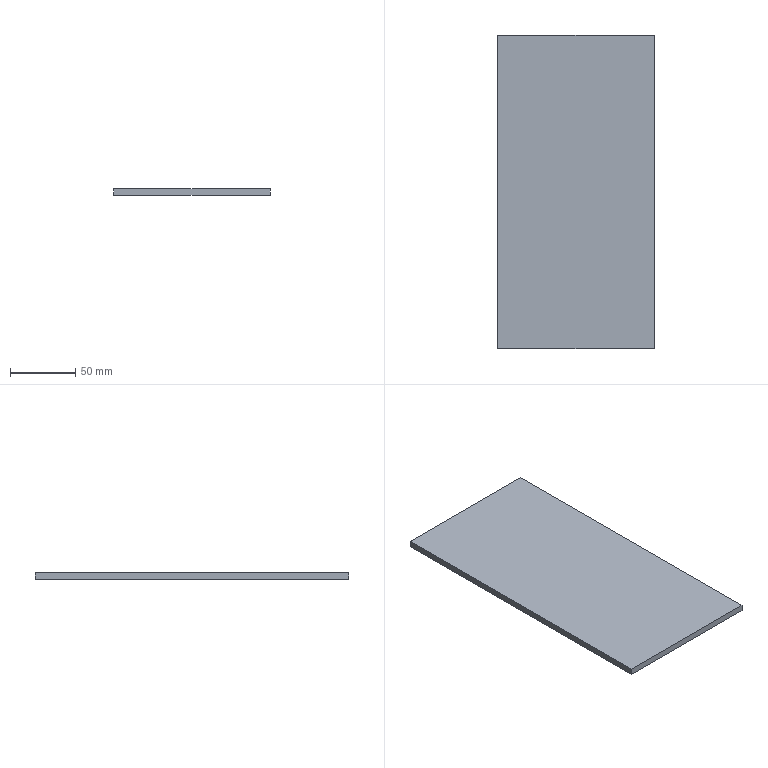Part | SolidWorks | features Extrusion 1 | 1 solid | 6 faces | box 120 x 240 x 5 mm | volume 144000 mm3 | plane 6
STEP:
#1=CARTESIAN_POINT('',(16.745,0.,0.));
#2=VERTEX_POINT('',#1);
#3=CARTESIAN_POINT('',(136.745,0.,0.));
#4=VERTEX_POINT('',#3);
#5=CARTESIAN_POINT('',(136.745,0.,0.));
#6=DIRECTION('',(1.,0.,0.));
#7=VECTOR('',#6,1000.);
#8=LINE('',#5,#7);
#9=EDGE_CURVE('',#2,#4,#8,.T.);
#10=ORIENTED_EDGE('',*,*,#9,.T.);
#11=CARTESIAN_POINT('',(136.745,0.,5.));
#12=VERTEX_POINT('',#11);
#13=CARTESIAN_POINT('',(136.745,0.,5.));
#14=DIRECTION('',(0.,0.,-1.));
#15=VECTOR('',#14,1000.);
#16=LINE('',#13,#15);
#17=EDGE_CURVE('',#12,#4,#16,.T.);
#18=ORIENTED_EDGE('',*,*,#17,.F.);
#19=CARTESIAN_POINT('',(16.745,0.,5.));
#20=VERTEX_POINT('',#19);
#21=CARTESIAN_POINT('',(136.745,0.,5.));
#22=DIRECTION('',(1.,0.,0.));
#23=VECTOR('',#22,1000.);
#24=LINE('',#21,#23);
#25=EDGE_CURVE('',#20,#12,#24,.T.);
#26=ORIENTED_EDGE('',*,*,#25,.F.);
#27=CARTESIAN_POINT('',(16.745,0.,5.));
#28=DIRECTION('',(0.,0.,-1.));
#29=VECTOR('',#28,1000.);
#30=LINE('',#27,#29);
#31=EDGE_CURVE('',#20,#2,#30,.T.);
#32=ORIENTED_EDGE('',*,*,#31,.T.);
#33=EDGE_LOOP('',(#10,#18,#26,#32));
#34=FACE_OUTER_BOUND('',#33,.T.);
#35=CARTESIAN_POINT('',(136.745,0.,5.));
#36=DIRECTION('',(0.,1.,0.));
#37=DIRECTION('',(0.,0.,1.));
#38=AXIS2_PLACEMENT_3D('',#35,#36,#37);
#39=PLANE('',#38);
#40=ADVANCED_FACE('',(#34),#39,.F.);
#41=CARTESIAN_POINT('',(136.745,240.,0.));
#42=VERTEX_POINT('',#41);
#43=CARTESIAN_POINT('',(136.745,240.,0.));
#44=DIRECTION('',(0.,1.,0.));
#45=VECTOR('',#44,1000.);
#46=LINE('',#43,#45);
#47=EDGE_CURVE('',#4,#42,#46,.T.);
#48=ORIENTED_EDGE('',*,*,#47,.T.);
#49=CARTESIAN_POINT('',(136.745,240.,5.));
#50=VERTEX_POINT('',#49);
#51=CARTESIAN_POINT('',(136.745,240.,5.));
#52=DIRECTION('',(0.,0.,-1.));
#53=VECTOR('',#52,1000.);
#54=LINE('',#51,#53);
#55=EDGE_CURVE('',#50,#42,#54,.T.);
#56=ORIENTED_EDGE('',*,*,#55,.F.);
#57=CARTESIAN_POINT('',(136.745,240.,5.));
#58=DIRECTION('',(0.,1.,0.));
#59=VECTOR('',#58,1000.);
#60=LINE('',#57,#59);
#61=EDGE_CURVE('',#12,#50,#60,.T.);
#62=ORIENTED_EDGE('',*,*,#61,.F.);
#63=ORIENTED_EDGE('',*,*,#17,.T.);
#64=EDGE_LOOP('',(#48,#56,#62,#63));
#65=FACE_OUTER_BOUND('',#64,.T.);
#66=CARTESIAN_POINT('',(136.745,240.,5.));
#67=DIRECTION('',(-1.,0.,0.));
#68=DIRECTION('',(0.,0.,1.));
#69=AXIS2_PLACEMENT_3D('',#66,#67,#68);
#70=PLANE('',#69);
#71=ADVANCED_FACE('',(#65),#70,.F.);
#72=CARTESIAN_POINT('',(16.745,240.,0.));
#73=VERTEX_POINT('',#72);
#74=CARTESIAN_POINT('',(16.745,240.,0.));
#75=DIRECTION('',(-1.,0.,0.));
#76=VECTOR('',#75,1000.);
#77=LINE('',#74,#76);
#78=EDGE_CURVE('',#42,#73,#77,.T.);
#79=ORIENTED_EDGE('',*,*,#78,.T.);
#80=CARTESIAN_POINT('',(16.745,240.,5.));
#81=VERTEX_POINT('',#80);
#82=CARTESIAN_POINT('',(16.745,240.,5.));
#83=DIRECTION('',(0.,0.,-1.));
#84=VECTOR('',#83,1000.);
#85=LINE('',#82,#84);
#86=EDGE_CURVE('',#81,#73,#85,.T.);
#87=ORIENTED_EDGE('',*,*,#86,.F.);
#88=CARTESIAN_POINT('',(16.745,240.,5.));
#89=DIRECTION('',(-1.,0.,0.));
#90=VECTOR('',#89,1000.);
#91=LINE('',#88,#90);
#92=EDGE_CURVE('',#50,#81,#91,.T.);
#93=ORIENTED_EDGE('',*,*,#92,.F.);
#94=ORIENTED_EDGE('',*,*,#55,.T.);
#95=EDGE_LOOP('',(#79,#87,#93,#94));
#96=FACE_OUTER_BOUND('',#95,.T.);
#97=CARTESIAN_POINT('',(16.745,240.,5.));
#98=DIRECTION('',(0.,-1.,0.));
#99=DIRECTION('',(0.,0.,-1.));
#100=AXIS2_PLACEMENT_3D('',#97,#98,#99);
#101=PLANE('',#100);
#102=ADVANCED_FACE('',(#96),#101,.F.);
#103=CARTESIAN_POINT('',(16.745,0.,0.));
#104=DIRECTION('',(0.,-1.,0.));
#105=VECTOR('',#104,1000.);
#106=LINE('',#103,#105);
#107=EDGE_CURVE('',#73,#2,#106,.T.);
#108=ORIENTED_EDGE('',*,*,#107,.T.);
#109=ORIENTED_EDGE('',*,*,#31,.F.);
#110=CARTESIAN_POINT('',(16.745,0.,5.));
#111=DIRECTION('',(0.,-1.,0.));
#112=VECTOR('',#111,1000.);
#113=LINE('',#110,#112);
#114=EDGE_CURVE('',#81,#20,#113,.T.);
#115=ORIENTED_EDGE('',*,*,#114,.F.);
#116=ORIENTED_EDGE('',*,*,#86,.T.);
#117=EDGE_LOOP('',(#108,#109,#115,#116));
#118=FACE_OUTER_BOUND('',#117,.T.);
#119=CARTESIAN_POINT('',(16.745,0.,5.));
#120=DIRECTION('',(1.,0.,0.));
#121=DIRECTION('',(0.,0.,-1.));
#122=AXIS2_PLACEMENT_3D('',#119,#120,#121);
#123=PLANE('',#122);
#124=ADVANCED_FACE('',(#118),#123,.F.);
#125=ORIENTED_EDGE('',*,*,#25,.T.);
#126=ORIENTED_EDGE('',*,*,#61,.T.);
#127=ORIENTED_EDGE('',*,*,#92,.T.);
#128=ORIENTED_EDGE('',*,*,#114,.T.);
#129=EDGE_LOOP('',(#125,#126,#127,#128));
#130=FACE_OUTER_BOUND('',#129,.T.);
#131=CARTESIAN_POINT('',(0.,0.,5.));
#132=DIRECTION('',(0.,0.,-1.));
#133=DIRECTION('',(-1.,0.,0.));
#134=AXIS2_PLACEMENT_3D('',#131,#132,#133);
#135=PLANE('',#134);
#136=ADVANCED_FACE('',(#130),#135,.F.);
#137=ORIENTED_EDGE('',*,*,#9,.F.);
#138=ORIENTED_EDGE('',*,*,#107,.F.);
#139=ORIENTED_EDGE('',*,*,#78,.F.);
#140=ORIENTED_EDGE('',*,*,#47,.F.);
#141=EDGE_LOOP('',(#137,#138,#139,#140));
#142=FACE_OUTER_BOUND('',#141,.T.);
#143=CARTESIAN_POINT('',(0.,0.,0.));
#144=DIRECTION('',(0.,0.,-1.));
#145=DIRECTION('',(-1.,0.,0.));
#146=AXIS2_PLACEMENT_3D('',#143,#144,#145);
#147=PLANE('',#146);
#148=ADVANCED_FACE('',(#142),#147,.T.);
#149=CLOSED_SHELL('',(#40,#71,#102,#124,#136,#148));
#150=MANIFOLD_SOLID_BREP('',#149);
#151=CARTESIAN_POINT('',(0.,0.,0.));
#152=DIRECTION('',(0.,0.,1.));
#153=DIRECTION('',(1.,0.,0.));
#154=AXIS2_PLACEMENT_3D('',#151,#152,#153);
#155=(LENGTH_UNIT()NAMED_UNIT(*)SI_UNIT(.MILLI.,.METRE.));
#156=UNCERTAINTY_MEASURE_WITH_UNIT(LENGTH_MEASURE(0.00001),#155,'','');
#157=(NAMED_UNIT(*)PLANE_ANGLE_UNIT()SI_UNIT($,.RADIAN.));
#158=(NAMED_UNIT(*)SI_UNIT($,.STERADIAN.)SOLID_ANGLE_UNIT());
#159=(GEOMETRIC_REPRESENTATION_CONTEXT(3)GLOBAL_UNCERTAINTY_ASSIGNED_CONTEXT((#156))GLOBAL_UNIT_ASSIGNED_CONTEXT((#155,#157,#158))REPRESENTATION_CONTEXT('',''));
#160=ADVANCED_BREP_SHAPE_REPRESENTATION('',(#150,#154),#159);